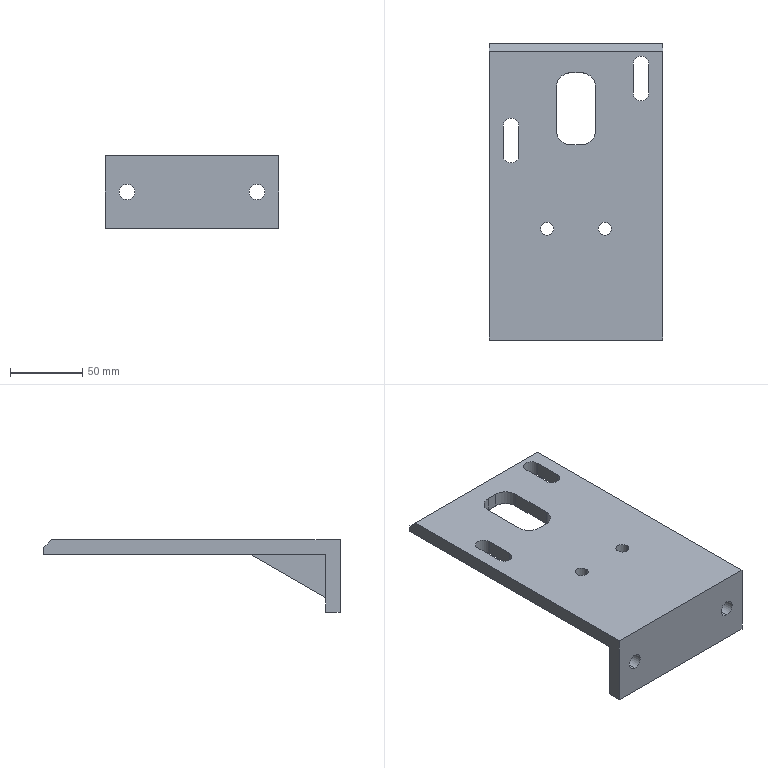NC program | NX | posted with a generic post | part box 120 x 205 x 50 mm
Whole program:
N10 G17 G21 G94 G90
(HOLE_MILLING_COPY_1 , TOOL : D6)
N12 T12 M6
N14 G54
N16 G17 G0 G90 X-45. Y0. B0. C0. S9500 M3
N18 G43 Z30. H12
N20 Z0.5
N22 G94 G3 X-46.2 Y1.2 R1.2 F1650.
N24 X-47.4 Y0. R1.2
N26 X-47.4 Y0. Z0. I2.4 J0.
N28 X-47.4 Y0. Z-0.5 I2.4 J0.
N30 X-47.4 Y0. Z-1. I2.4 J0.
N32 X-47.4 Y0. Z-1.5 I2.4 J0.
N34 X-47.4 Y0. Z-2. I2.4 J0.
N36 X-47.4 Y0. Z-2.5 I2.4 J0.
N38 X-47.4 Y0. Z-3. I2.4 J0.
N40 X-47.4 Y0. Z-3.5 I2.4 J0.
N42 X-47.4 Y0. Z-4. I2.4 J0.
N44 X-47.4 Y0. Z-4.5 I2.4 J0.
N46 X-47.4 Y0. Z-5. I2.4 J0.
N48 X-47.4 Y0. Z-5.5 I2.4 J0.
N50 X-47.4 Y0. Z-6. I2.4 J0.
N52 X-47.4 Y0. Z-6.5 I2.4 J0.
N54 X-47.4 Y0. Z-7. I2.4 J0.
N56 X-47.4 Y0. Z-7.5 I2.4 J0.
N58 X-47.4 Y0. Z-8. I2.4 J0.
N60 X-47.4 Y0. Z-8.5 I2.4 J0.
N62 X-47.4 Y0. Z-9. I2.4 J0.
N64 X-47.4 Y0. Z-9.5 I2.4 J0.
N66 X-47.4 Y0. Z-10. I2.4 J0.
N68 X-45. Y-2.4 R2.4
N70 X-47.4 Y0. R-2.4
N72 X-46.2 Y-1.2 R1.2
N74 X-45. Y0. R1.2
N76 G0 Z30.
N78 X45.
N80 Z0.5
N82 G3 X43.8 Y1.2 R1.2
N84 X42.6 Y0. R1.2
N86 X42.6 Y0. Z0. I2.4 J0.
N88 X42.6 Y0. Z-0.5 I2.4 J0.
N90 X42.6 Y0. Z-1. I2.4 J0.
N92 X42.6 Y0. Z-1.5 I2.4 J0.
N94 X42.6 Y0. Z-2. I2.4 J0.
N96 X42.6 Y0. Z-2.5 I2.4 J0.
N98 X42.6 Y0. Z-3. I2.4 J0.
N100 X42.6 Y0. Z-3.5 I2.4 J0.
N102 X42.6 Y0. Z-4. I2.4 J0.
N104 X42.6 Y0. Z-4.5 I2.4 J0.
N106 X42.6 Y0. Z-5. I2.4 J0.
N108 X42.6 Y0. Z-5.5 I2.4 J0.
N110 X42.6 Y0. Z-6. I2.4 J0.
N112 X42.6 Y0. Z-6.5 I2.4 J0.
N114 X42.6 Y0. Z-7. I2.4 J0.
N116 X42.6 Y0. Z-7.5 I2.4 J0.
N118 X42.6 Y0. Z-8. I2.4 J0.
N120 X42.6 Y0. Z-8.5 I2.4 J0.
N122 X42.6 Y0. Z-9. I2.4 J0.
N124 X42.6 Y0. Z-9.5 I2.4 J0.
N126 X42.6 Y0. Z-10. I2.4 J0.
N128 X45. Y-2.4 R2.4
N130 X42.6 Y0. R-2.4
N132 X43.8 Y-1.2 R1.2
N134 X45. Y0. R1.2
N136 G0 Z30.
N138 M5
(PLANAR_MILL_COPY_COPY_COPY_COPY_COPY_COPY_1_COPY_1 , TOOL : D6A45)
N140 T01 M6
N142 G54
N144 G17 G0 G90 X-48.07 Y1.461 B0. C0. S9500 M3
N146 G43 Z30. H1
N148 Z0.5
N150 G94 G1 Z-1. F1250.
N152 X-49.1 Y0.866
N154 G3 X-49.6 Y0. R1.
N156 X-45. Y-4.6 R4.6
N158 X-49.6 Y0. R-4.6
N160 X-49.1 Y-0.866 R1.
N162 G1 X-48.07 Y-1.461
N164 Z0.5
N166 G0 Z30.
N168 X48.07
N170 Z0.5
N172 G1 Z-1.
N174 X49.1 Y-0.866
N176 G3 X49.6 Y0. R1.
N178 X45. Y4.6 R4.6
N180 X49.6 Y0. R-4.6
N182 X49.1 Y0.866 R1.
N184 G1 X48.07 Y1.461
N186 Z0.5
N188 G0 Z30.
N190 M5
(刀补 , TOOL : D6)
N192 T12 M6
N194 G54
N196 G17 G0 G90 X-45. Y0. B0. C0. S9500 M3
N198 G43 Z30. H12
N200 Z0.5
N202 G41 G94 G1 X-44.991 Y0.1 F1000. D12
N204 G3 X-47.45 Y0. R1.232
N206 X-47.45 Y0. Z-1.5 I2.45 J0.
N208 X-47.45 Y0. Z-3.5 I2.45 J0.
N210 X-47.45 Y0. Z-5.5 I2.45 J0.
N212 X-47.45 Y0. Z-7.5 I2.45 J0.
N214 X-47.45 Y0. Z-9.5 I2.45 J0.
N216 X-45. Y-2.45 Z-10. R2.45
N218 X-42.55 Y0. R2.45
N220 X-45. Y-2.45 R-2.45
N222 X-44.9 Y0.009 R1.232
N224 G40
N226 G1 X-45. Y0.
N228 G0 Z30.
N230 X45.
N232 Z0.5
N234 G41 G1 X45.009 Y0.1
N236 G3 X42.55 Y0. R1.232
N238 X42.55 Y0. Z-1.5 I2.45 J0.
N240 X42.55 Y0. Z-3.5 I2.45 J0.
N242 X42.55 Y0. Z-5.5 I2.45 J0.
N244 X42.55 Y0. Z-7.5 I2.45 J0.
N246 X42.55 Y0. Z-9.5 I2.45 J0.
N248 X45. Y-2.45 Z-10. R2.45
N250 X47.45 Y0. R2.45
N252 X45. Y-2.45 R-2.45
N254 X45.1 Y0.009 R1.232
N256 G40
N258 G1 X45. Y0.
N260 G0 Z30.
N262 M5
N264 M2